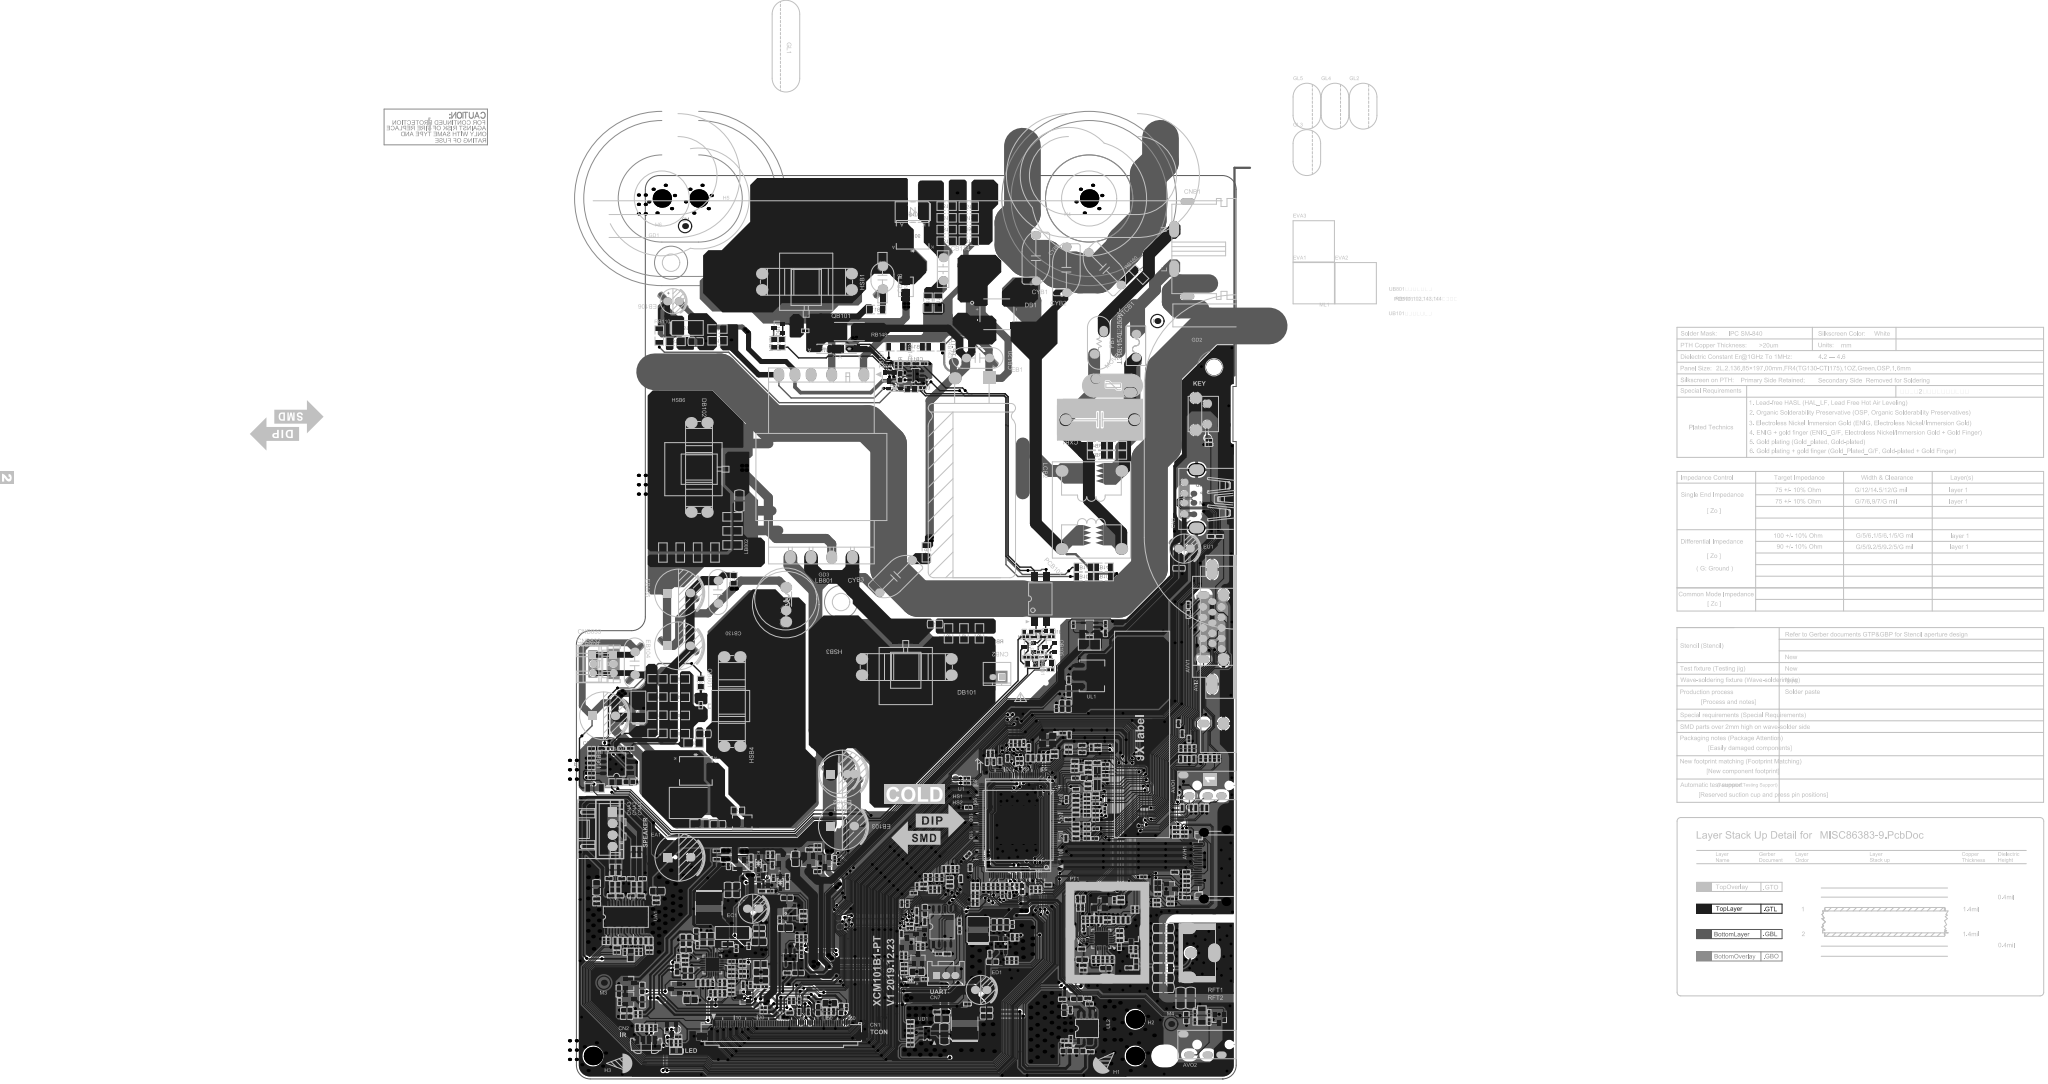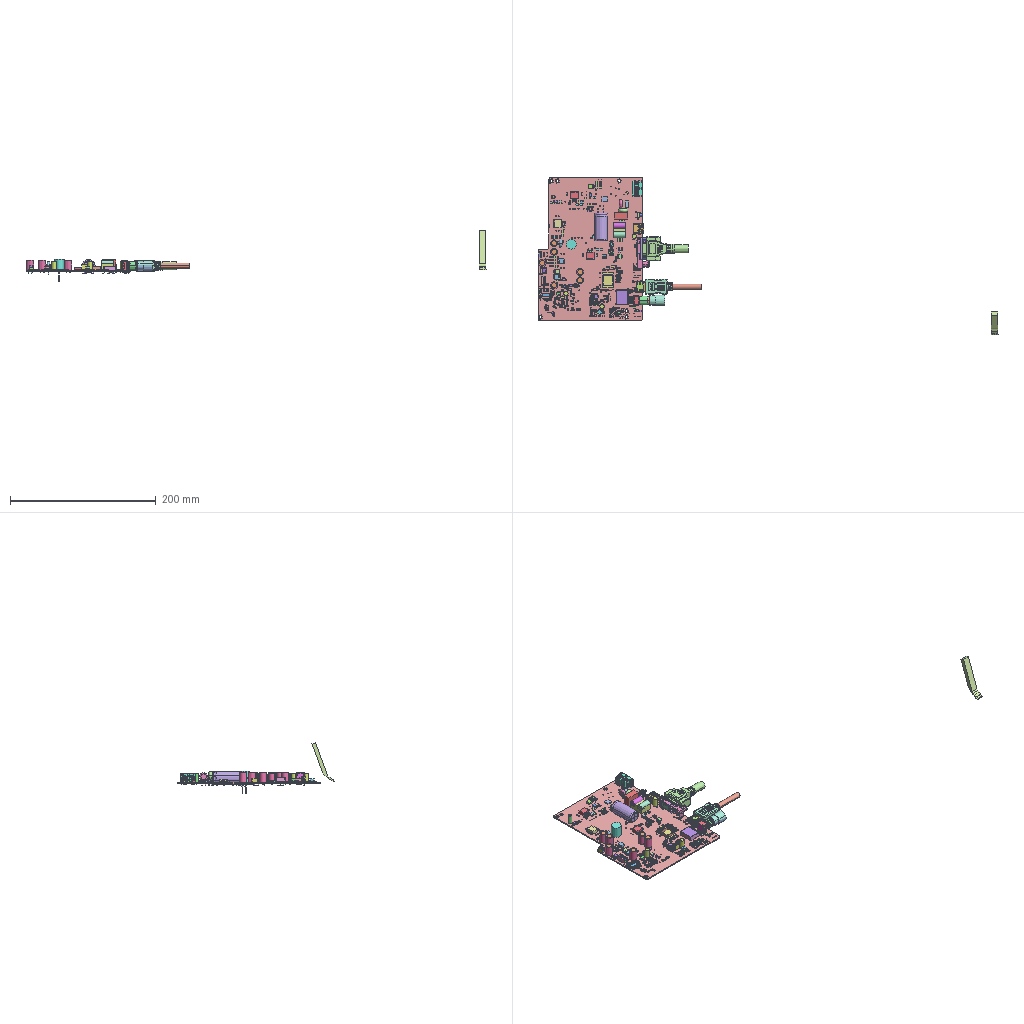Circuit board layout | Altium Designer | box 631.6 x 216.7 x 69.7 mm
Part placement, first 370 of 744 lines:
Designator,Comment,Layer,Footprint,Center-X(mm),Center-Y(mm),Rotation
ML1,NC/Mylar sheet,XXXXXXXXXXXXXXX,(85+6)×(123.5+6)×0.43mm,SE42B,black,TopLayer,Mylar,-883.787,-746.906,90
EVA6,NC/7×7×3mm-C-4305 fire-retardant foam-black,BottomLayer,EVA(7*7*3),-883.787,-746.906,180
EVA5,NC/7×7×3mm-C-4305 fire-retardant foam-black,BottomLayer,EVA(7*7*3),-883.787,-746.906,180
EVA4,NC/7×7×3mm-C-4305 fire-retardant foam-black,BottomLayer,EVA(7*7*3),-883.787,-746.906,180
RV23,NC/Thick film resistor,RES,1/16W,0ohm,±1%,0402,SMD,TopLayer,R0402,-3.759,69.901,90
RV22,NC/Thick film resistor,RES,1/16W,0ohm,±1%,0402,SMD,TopLayer,R0402,-5.69,69.901,90
DK2,NC/TVS diode,DIO ESD,3pF,58V,0402,SMD,SDV1005H260C030YPTF,Sunlord,TopLayer,DIODE-S0402,-14.275,38.151,180
CVBS_IN/OUT,TEST,BottomLayer,TP,-10.108,59.398,90
OE1,TEST,BottomLayer,TP,-86.335,33.172,180
RC36,Thick film resistor,RES,1/16W,10ohm,±1%,0402,SMD,TopLayer,R0402,-99.365,34.747,270
RG5,Thick film resistor,RES,1/16W,0ohm,±1%,0402,SMD,TopLayer,R0402,-129.692,14.097,270
H5,Location hole,TopLayer,ASSE4.0C-3,-117.05,191.85,0
CT5,NC/10uF-0603-X5R-±20%-6.3V,TopLayer,C0603,-33.517,26.012,360
H6,Location hole,TopLayer,ASSE4.0C-3,-125.05,191.85,0
UR1,NC/SGM810-SXN3L,TopLayer,SO-23-1,-68.801,31.533,90
RV21,Thick film resistor,RES,1/16W,0ohm,±1%,0402,SMD,TopLayer,R0402,-60.223,34.29,90
RV20,Thick film resistor,RES,1/16W,0ohm,±1%,0402,SMD,TopLayer,R0402,-60.198,32.41,90
RR6,NC/0ohm-0402-±5%-1/16W,TopLayer,R0402,-72.847,31.598,270
RR5,NC/0ohm-0402-±5%-1/16W,TopLayer,R0402,-69.207,28.84,270
RR2,NC/100Kohm-0402-±5%-1/16W,TopLayer,R0402,-71.044,33.757,360
RR1,NC/1Kohm-0402-±5%-1/16W,TopLayer,R0402,-71.044,32.842,180
RA38,NC/100Kohm-0402-±5%-1/16W,TopLayer,R0402,-72.83,26.909,90
RA31,NC/NC/470Kohm-0402-±5%-1/16W,TopLayer,R0402,-67.759,21.754,180
RA19,NC/33Kohm-0402-±5%-1/16W,TopLayer,R0402,-72.28,24.98,180
RA18,NC/33Kohm-0402-±5%-1/16W,TopLayer,R0402,-72.28,23.125,180
RA16,NC/2Kohm-0402-±1%-1/16W,TopLayer,R0402,-72.28,24.04,360
RA10,NC/2K2ohm-0402-±5%-1/16W,TopLayer,R0402,-71.89,26.897,90
QA3,NC/LMBT3904LT1G,TopLayer,SOT-23,-71.696,29.704,180
QA2,NC/LMBT3906LT1G,TopLayer,SOT-23,-69.258,26.148,180
HS2,NC/Heat sink,15.0×15.0×5.0mm,AL1060H-24,black,high-emissivity paint,stamped with bend,no press-fit legs,YT,TopLayer,HS(15X15X5)-S,-883.787,-746.906,0
H3,Location hole,TopLayer,ASSE4.0C-3,-139.831,4.85,0
DV8,NC/SFI0402-240E-2R5PP-LF,TopLayer,DIODE-S0402,-17.29,37.952,360
DV7,NC/SFI0402-240E-2R5PP-LF,TopLayer,DIODE-S0402,-17.306,38.969,360
DV6,NC/SFI0402-240E-2R5PP-LF,TopLayer,DIODE-S0402,-6.655,69.901,270
DV5,NC/SFI0402-240E-2R5PP-LF,TopLayer,DIODE-S0402,-4.724,69.901,270
DR1,NC/AVLC18S02003,TopLayer,DIODE-S0402,-59.957,43.612,90
CV23,NC/33pF-0402-NPO-±5%-50V,TopLayer,C0402,-11.748,75.285,270
CV22,NC/33pF-0402-NPO-±5%-50V,TopLayer,C0402,-12.56,77.47,270
CV21,NC/33pF-0402-NPO-±5%-50V,TopLayer,C0402,-10.44,101.289,270
CV20,NC/33pF-0402-NPO-±5%-50V,TopLayer,C0402,-9.195,69.781,90
CV19,NC/33pF-0402-NPO-±5%-50V,TopLayer,C0402,-9.155,72.056,90
CT2,10uF-0603-X5R-±20%-6.3V,TopLayer,C0603,-28.386,24.132,180
CR1,NC/1uF-0402-X5R-±20%-16V,TopLayer,C0402,-68.191,28.866,270
CO77,NC/10uF-0603-X5R-±20%-6.3V,TopLayer,C0603,-10.846,13.365,270
CA36,NC/10uF-0805-X5R-±20%-16V,TopLayer,C0805,-69.448,23.398,360
RT78,NC/,TopLayer,R0402SC,-33.419,37.384,90
RT77,NC/,TopLayer,R0402SC,-34.337,37.384,90
CT71,NC/30pF-0402-NPO-±5%-50V,TopLayer,C0402,-33.266,39.229,270
CT70,NC/30pF-0402-NPO-±5%-50V,TopLayer,C0402,-34.52,39.205,90
CF5,NC/0ohm-0402-PCB,TopLayer,R0402SC,-25.11,39.563,180
CF14,NC/4.7pF-0402-NPO-±5%-50V,TopLayer,C0402,-25.11,38.547,180
LF1,1000pF-0402-X7R-±10%-50V,TopLayer,L0402,-26.52,38.966,90
CT15,NC/8pF-0402-NPO-±5%-50V,TopLayer,C0402,-30.414,34.711,270
CT14,NC/8pF-0402-NPO-±5%-50V,TopLayer,C0402,-31.379,34.736,90
YT1,NC/Passive standard-package crystal oscillator,SPXO,24MHz,±20ppm,16pF,3.2×2.5,SMD,SMD3225 24.000MHZ,JWT,TopLayer,XTAL-S-10,-29.758,38.102,360
RT18,Thick film resistor,RES,1/16W,10Kohm,±1%,0402,SMD,TopLayer,R0402,-32.344,34.724,90
RT11,Thick film resistor,RES,1/16W,1.8Kohm,±1%,0402,SMD,TopLayer,R0402,-26.642,34.699,270
RT6,Thick film resistor,RES,1/16W,33ohm,±1%,0402,SMD,TopLayer,R0402,-21.581,36.946,90
RT5,Thick film resistor,RES,1/16W,33ohm,±1%,0402,SMD,TopLayer,R0402,-22.496,36.946,90
RT2,Thick film resistor,RES,1/16W,100ohm,±1%,0402,SMD,TopLayer,R0402,-33.258,34.736,90
LT12,Ferrite bead,BEAD,120ohm,0402,800mA,SMD,TP,CBM100505U121T,FH,TopLayer,L0402,-33.263,23.726,360
LT11,NC/SDCL1005CR27JTDF(Sunlord),TopLayer,L0402,-22.146,26.838,180
LT10,SDCL1005CR18JTDF(180nH-0402±5%-C),TopLayer,L0402,-25.346,31.282,360
LT9,NC/SDCL1608CR22JT(F),TopLayer,L0603,-21.75,25.04,270
LT8,GZ1005U102CTF(1000ohm-300mA),TopLayer,L0402,-25.346,30.177,360
LT6,GZ1005U102CTF(1000ohm-300mA),TopLayer,L0402,-25.435,28.818,270
LT3,Thick film resistor,RES,1/16W,0ohm,±1%,0402,SMD,TopLayer,L0402,-22.907,28.272,90
LT2,GZ1005U102CTF(1000ohm-300mA),TopLayer,L0402,-29.029,26.062,270
LT1,Multilayer inductor,HF Inductor,68nH,±5%,0402,SMD,SDCL1005C68NJTDF,Sunlord,TopLayer,L0402,-28.064,26.062,90
DT1,Switching diode,DIO SW D2,200mA,100V,SOT-23,SMD,BAV99,YJ,TopLayer,SO-23,-22.839,30.813,360
CT29,6800pF-0402-X7R-±10%-50V,TopLayer,C0402,-28.026,35.13,360
CT27,Ceramic capacitor,CAP MC,16V,0.1uF,±10%,X7R,0402,SMD,TP,TopLayer,C0402,-29.436,34.698,90
CT26,330pF-0402-NPO-±5%-50V,TopLayer,C0402,-28.026,34.203,360
CT25,Ceramic capacitor,CAP MC,16V,0.1uF,±10%,X7R,0402,SMD,TP,TopLayer,C0402,-25.677,34.648,90
CT21,0.047uF-0402-X7R-±10%-16V,TopLayer,C0402,-25.372,32.348,360
CT18,Ceramic capacitor,CAP MC,16V,0.1uF,±10%,X7R,0402,SMD,TP,TopLayer,C0402,-33.614,28.323,360
CT17,NC/180pF-0402-NPO-±5%-50V,TopLayer,C0402,-23.374,24.216,180
CT13,NC/1.2pF-0402-NPO-±0.25pf-50V,TopLayer,C0402,-21.831,28.24,90
CT12,0.022uF-0402-X7R-±10%-16V,TopLayer,C0402,-31.067,26.062,270
CT11,0.022uF-0402-X7R-±10%-16V,TopLayer,C0402,-29.987,26.063,90
CT9,Ceramic capacitor,CAP MC,16V,0.1uF,±10%,X7R,0402,SMD,TP,TopLayer,C0402,-26.997,26.062,270
CT8,Ceramic capacitor,CAP MC,50V,22pF,±5%,NPO,0402,SMD,TP,TopLayer,C0402,-23.53,34.648,270
CT7,Ceramic capacitor,CAP MC,50V,22pF,±5%,NPO,0402,SMD,TP,TopLayer,C0402,-24.597,34.648,270
CT6,Ceramic capacitor,CAP MC,16V,0.1uF,±10%,X7R,0402,SMD,TP,TopLayer,C0402,-33.289,24.767,180
CT1,Ceramic capacitor,CAP MC,16V,0.1uF,±10%,X7R,0402,SMD,TP,TopLayer,C0402,-33.225,32.933,90
UT1,Silicon tuner IC,IC Si Tuner,QFN24,SMD,R842,Rafael,TopLayer,QFN24/0.5-3,-29.36,30.57,180
RT9,NC/430ohm-0402-±5%-1/16W,TopLayer,R0402,-31.534,72.238,90
RT8,NC/,TopLayer,R0402SC,-30.163,72.721,180
RT7,NC/,TopLayer,R0402SC,-30.163,71.794,180
CT24,30pF-0402-NPO-±5%-50V,TopLayer,C0402,-33.521,72.721,180
CT23,Ceramic capacitor,CAP MC,16V,0.1uF,±10%,X7R,0402,SMD,TP,TopLayer,C0402,-36.487,72.371,180
CT20,Ceramic capacitor,CAP MC,16V,0.1uF,±10%,X7R,0402,SMD,TP,TopLayer,C0402,-36.487,71.26,180
CT10,30pF-0402-NPO-±5%-50V,TopLayer,C0402,-33.521,71.184,360
5V_STB,TEST,BottomLayer,TP,-74.651,18.466,90
RG62,Thick film resistor,RES,1/16W,0ohm,±1%,0402,SMD,TopLayer,R0402,-69.469,41.986,270
RG60,NC/33ohm-0402-±5%-1/16W,TopLayer,R0402,-58.611,64.529,180
RG59,Thick film resistor,RES,1/16W,0ohm,±1%,0402,SMD,TopLayer,R0402,-70.18,40.538,180
RG15,12Kohm-0402-±1%-1/16W,TopLayer,R0402,-121.405,26.307,270
RG14,Thick film resistor,RES,1/16W,3Kohm,±1%,0402,SMD,TopLayer,R0402,-113.925,20.955,90
RG13,Thick film resistor,RES,1/16W,39Kohm,±1%,0402,SMD,TopLayer,R0402,-109.839,25.618,180
RG12,NC/Thick film resistor,RES,1/16W,10Kohm,±1%,0402,SMD,TopLayer,R0402,-95.123,14.599,270
CG22,NC/1uF-0603-X5R-±10%-50V,TopLayer,C0603,-103.81,31.521,360
Y1,Passive crystal oscillator,SPXO,24MHz,±10ppm,12pF,SMD3225,SMD,SX32Y024000BC1T-Z,TKD,TopLayer,XTAL-S-3,-41.006,73.97,180
XCM101B1-PT,PCB_NAME,TopLayer,PCB_NAME,-76.708,16.002,180
VON,TEST,BottomLayer,TP,-124.904,17.221,180
VOFF,TEST,BottomLayer,TP,-104.623,16.205,180
VMID/SDA,TEST,BottomLayer,TP,-61.151,65.532,90
VMID/SCL,TEST,BottomLayer,TP,-58.814,64.529,180
USB_5V,TEST,BottomLayer,TP,-9.31,123.13,180
USB0_DP,TEST,BottomLayer,TP,-9.31,127.63,180
USB0_DM,TEST,BottomLayer,TP,-9.31,125.63,180
UL3,LDO IC,IC LDO,0.3A,3.3V,6V,SOT23-5,SMD,LC1463CB5ATR33,Leadchip,TopLayer,SOP23-5-1,-97.079,26.454,180
UC4,Operational amplifier,AMP,1,9MHz,SOT-23-5,SMD,SGM8425AYN5G/TR,SGMICRO,TopLayer,SOT-23-5,-97.079,36.411,360
UC2,Tcon driver IC,IC Tcon  Driver,VQFN-24L,SMD,ANX6732AAQX,ANAX,TopLayer,QFN24/0.5-5,-114.014,24.973,360
UC1,Regulator IC,IC Regulator,2.50V,0.4%,SOT-23,SMD,BR431M-A,Blue Rocket,TopLayer,SO-23-1,-107.112,17.843,90
TVCOM,TEST,BottomLayer,TP,-96.203,15.989,180
TP,TEST,BottomLayer,TP,-92.786,12.357,180
SK1,Tact switch,Tact Switch,160±50gf,7.0×10.3×7.0mm,DIP,106520070,VAST,TopLayer,KEY-HD-6,-7.6,145,90
RM12,Thick film resistor,RES,1/16W,100Kohm,±1%,0402,SMD,TopLayer,R0402,-102.565,45.999,90
RL51,Thick film resistor,RES,1/16W,10Kohm,±1%,0402,SMD,TopLayer,R0402,-94.64,30.632,270
RL50,NC/10Kohm-0402-±5%-1/16W,TopLayer,R0402,-94.628,28.892,90
RL7,Thick film resistor,RES,1/16W,4.7Kohm,±1%,0402,SMD,TopLayer,R0402,-93.726,30.632,270
RL3,NC/Thick film resistor,RES,1/16W,4.7Kohm,±5%,0402,SMD,TopLayer,R0402,-95.555,30.632,270
RGV1,NC/0ohm-0402-±5%-1/16W,TopLayer,R0402,-71.564,38.227,270
RG78,NC/0ohm-0402-PCB,TopLayer,R0402SC,-72.784,38.227,270
RG48,Thick film resistor,RES,1/16W,0ohm,±1%,0402,SMD,TopLayer,R0402,-102.616,20.117,360
RG46,NC/0ohm-0402-±5%-1/16W,TopLayer,R0402,-66.523,41.3,270
RG43,Thick film resistor,RES,1/16W,0ohm,±1%,0402,SMD,TopLayer,R0402,-97.257,17.031,270
RG41,NC/0ohm-0402-±5%-1/16W,TopLayer,R0402,-84.823,15.672,270
RG39,Thick film resistor,RES,1/16W,0ohm,±1%,0402,SMD,TopLayer,R0402,-89.56,14.707,90
RG26,NC/0ohm-0402-PCB,TopLayer,R0402SC,-64.694,41.3,270
RG25,NC/0ohm-0402-±5%-1/16W,TopLayer,R0402,-68.047,41.478,180
RC35,10Kohm-0402-±1%-1/16W,TopLayer,R0402,-94.209,34.493,360
RC33,NC/0ohm-0402-±5%-1/16W,TopLayer,R0402,-102.845,14.63,360
RC32,Thick film resistor,RES,1/16W,0ohm,±1%,0402,SMD,TopLayer,R0402,-102.845,15.545,180
RC31,10Kohm-0402-±1%-1/16W,TopLayer,R0402,-94.221,36.551,180
RC27,Thick film resistor,RES,1/16W,47Kohm,±1%,0402,SMD,TopLayer,R0402,-130.683,14.097,270
RC24,Thick film resistor,RES,1/16W,10Kohm,±1%,0402,SMD,TopLayer,R0402,-119.507,18.694,180
RC23,NC/0ohm-0402-±5%-1/16W,TopLayer,R0402,-134.212,16.803,270
RC20,Thick film resistor,RES,1/16W,0ohm,±1%,0402,SMD,TopLayer,R0402,-113.055,49.733,180
RC19,NC/0ohm-0402-±5%-1/16W,TopLayer,R0402,-113.055,47.904,360
RC18,Thick film resistor,RES,1/16W,47Kohm,±1%,0402,SMD,TopLayer,R0402,-106.096,29.02,90
RC15,Thick film resistor,RES,1/16W,47Kohm,±1%,0402,SMD,TopLayer,R0402,-109.884,23.385,360
RC14,Thick film resistor,RES,1/16W,4.7ohm,±1%,0402,SMD,TopLayer,R0402,-109.88,20.304,360
RC13,Thick film resistor,RES,1/16W,51Kohm,±1%,0402,SMD,TopLayer,R0402,-109.884,24.401,360
RC12,Thick film resistor,RES,1/16W,33Kohm,±1%,0402,SMD,TopLayer,R0402,-109.884,22.471,180
RC10,Thick film resistor,RES,1/16W,100Kohm,±1%,0402,SMD,TopLayer,R0402,-109.893,19.393,360
RC8,NC/0ohm-0402-PCB,TopLayer,R0402SC,-119.945,24.948,360
RC4,NC/0ohm-0402-PCB,TopLayer,R0402SC,-107.29,20.523,90
RC3,Thick film resistor,RES,1/16W,1.8Kohm,±1%,0402,SMD,TopLayer,R0402,-105.715,20.523,270
RC2,12Kohm-0402-±1%-1/16W,TopLayer,R0402,-104.343,20.117,360
RC1,33ohm-0805-±5%-1/8W,TopLayer,R0805,-103.53,25.044,180
QM7,MOSFET,PMOS,-4.3A,-30V,0.048ohm@ID=-3A@VGS=-4.5V,SOT-23-3L,NCE3407AY,NCEPOWER,TopLayer,SOT-23-1,-108.013,46.532,360
POL,TEST,BottomLayer,TP,-94.767,12.383,180
NO DOLBY,NO DOLBY,BottomLayer,NO_DOLBY-SILK,-883.787,-746.906,180
LC1,Power inductor,Power Inductor,10uH,±10%,2A,0.3×1P,DR5.8×4.5,SMD,CKO54-10uH/K,CK,TopLayer,L(5.8*4.5)-S,-114.795,37.224,90
GREF,TEST,BottomLayer,TP,-92.024,15.926,180
EC1,Aluminium electrolytic capacitor,CAP AL,35V,100uF,±20%,LD,KF,P,2.5mm,6.3×11,DIP,TP,CapXon,TopLayer,EC(6.3*11)-V-2.5,-105.219,36.678,360
DM3,NC/Switching diode,DIO SW S,150mA,75V,SOD-323,SMD,1N4148WS,YJ,TopLayer,DIODE-S-12,-103.988,46.977,270
DK20,WEJT61RC-871-red,TopLayer,DIODE-S0603,-121.906,6.094,360
DC4,Switching diode,DIO SW D2,200mA,100V,SOT-23,SMD,BAV99,YJ,TopLayer,SO-23,-132.014,17.368,90
DC3,Switching diode,DIO SW D2,200mA,100V,SOT-23,SMD,BAV99,YJ,TopLayer,SO-23,-132.002,20.816,90
DC2,Switching diode,DIO SW D2,200mA,100V,SOT-23,SMD,BAV99,YJ,TopLayer,SO-23,-122.092,19.704,270
DC1,Schottky diode,DIO SBD S,1A,40V,DO-214AC,SMD,SS14W,WILLAS,TopLayer,DIODE-S-1,-109.576,31.826,360
CU6,NC/0ohm-0402-PCB,TopLayer,R0402SC,-53.95,70.907,270
CU5,NC/0ohm-0402-PCB,TopLayer,R0402SC,-53.035,70.907,270
CPV,TEST,BottomLayer,TP,-71.044,33.236,180
CPV2,TEST,BottomLayer,TP,-85.001,12.383,180
CN2,IR receiver transistor,IR Receriver,2.7-5.5V,37.9KHz,SMD,SIRAB39R1,SL,TopLayer,REMOTE-HS-1,-128.4,8.505,0
CN1,FFC connector,FFC connector,60Pin,D0.5,Bottom,lock,SMD,0.5-22-60PBX-P,XFE,TopLayer,FFC60H/0.5S-11,-99,10.727,360
CM11,Ceramic capacitor,CAP MC,16V,0.22uF,±20%,X5R,0402,SMD,TP,TopLayer,C0402,-105.588,48.197,90
CM10,NC/0.022uF-0402-X7R-±10%-50V,TopLayer,C0402,-105.55,46.304,90
CL16,Ceramic capacitor,CAP MC,16V,0.1uF,±10%,X7R,0402,SMD,TP,TopLayer,C0402,-94.615,27.114,270
CG16,Ceramic capacitor,CAP MC,50V,33pF,±5%,NPO,0402,SMD,TP,TopLayer,C0402,-108.814,28.435,90
CC51,1uF-0402-X5R-±20%-6.3V,TopLayer,C0402,-97.739,23.114,360
CC50,NC/10uF-0603-X5R-±20%-6.3V,TopLayer,C0603,-95.352,23.114,360
CC43,10uF-0805-X5R-±20%-16V,TopLayer,C0805,-98.12,32.982,180
CC42,Ceramic capacitor,CAP MC,16V,0.1uF,±10%,X7R,0402,SMD,TP,TopLayer,C0402,-94.208,35.496,360
CC38,Ceramic capacitor,CAP MC,50V,0.1uF,±10%,X7R,0603,SMD,TP,TopLayer,C0603,-97.777,39.484,180
CC34,Ceramic capacitor,CAP MC,50V,0.1uF,±10%,X7R,0603,SMD,TP,TopLayer,C0603,-132.651,13.614,360
CC33,1uF-0603-X5R-±10%-50V,TopLayer,C0603,-132.639,15.011,360
CC32,NC/33pF-0402-NPO-±5%-50V,TopLayer,C0402,-113.392,18.669,270
CC31,Ceramic capacitor,CAP MC,50V,0.1uF,±10%,X7R,0603,SMD,TP,TopLayer,C0603,-129.235,16.815,90
CC30,NC/10uF-0805-X5R-±20%-16V,TopLayer,C0805,-118.77,17.259,360
CC29,10uF-0805-X5R-±20%-16V,TopLayer,C0805,-88.468,16.485,360
CC27,Ceramic capacitor,CAP MC,50V,0.1uF,±10%,X7R,0603,SMD,TP,TopLayer,C0603,-129.235,19.761,270
CC26,NC/33pF-0402-NPO-±5%-50V,TopLayer,C0402,-111.36,18.669,270
CC25,NC/33pF-0402-NPO-±5%-50V,TopLayer,C0402,-107.449,25.645,360
CC24,Ceramic capacitor,CAP MC,16V,0.1uF,±10%,X7R,0402,SMD,TP,TopLayer,C0402,-117.129,20.937,270
CC23,NC/0.1uF-0402-X5R-±20%-16V,TopLayer,C0402,-107.444,22.396,180
CC21,Ceramic capacitor,CAP MC,50V,1000pF,±10%,X7R,0402,SMD,TP,TopLayer,C0402,-107.444,23.463,360
CC20,Ceramic capacitor,CAP MC,25V,1uF,±10%,X7R,0603,SMD,TP,TopLayer,C0603,-103.81,32.944,360
CC19,Ceramic capacitor,CAP MC,25V,10uF,±10%,X5R,0805,SMD,TP,TopLayer,C0805,-103.835,29.909,360
CC18,1uF-0402-X5R-±20%-6.3V,TopLayer,C0402,-109.884,21.302,180
CC17,1uF-0402-X5R-±20%-6.3V,TopLayer,C0402,-111.36,20.955,90
CC15,1uF-0402-X5R-±20%-6.3V,TopLayer,C0402,-114.98,20.955,270
CC13,NC/0.1uF-0402-X5R-±20%-16V,TopLayer,C0402,-110.503,46.495,270
CC12,NC/Ceramic capacitor,CAP MC,16V,10uF,±20%,X5R,0805,SMD,TP,TopLayer,C0805,-110.582,41.219,90
CC11,Ceramic capacitor,CAP MC,50V,0.1uF,±10%,X7R,0603,SMD,TP,TopLayer,C0603,-119.698,28.092,180
CC10,Ceramic capacitor,CAP MC,50V,0.1uF,±10%,X7R,0603,SMD,TP,TopLayer,C0603,-120.421,30.226,90
CC9,NC/0.1uF-0603-X7R-±10%-50V,TopLayer,C0603,-118.999,30.226,90
CC8,Ceramic capacitor,CAP MC,16V,10uF,±20%,X5R,0805,SMD,TP,TopLayer,C0805,-108.753,41.219,90
CC7,Ceramic capacitor,CAP MC,50V,0.1uF,±10%,X7R,0603,SMD,TP,TopLayer,C0603,-120.053,23.05,270
CC5,Ceramic capacitor,CAP MC,16V,2.2uF,±10%,X5R,0603,SMD,TP,TopLayer,C0603,-121.672,23.919,270
CC4,Ceramic capacitor,CAP MC,25V,1uF,±10%,X7R,0603,SMD,TP,TopLayer,C0603,-118.681,23.05,90
CC2,Ceramic capacitor,CAP MC,25V,10uF,±10%,X5R,0805,SMD,TP,TopLayer,C0805,-103.454,23.312,180
CC1,NC/Ceramic capacitor,CAP MC,25V,10uF,±10%,X5R,0805,SMD,TP,TopLayer,C0805,-103.454,21.483,180
3V3_TUNER,TEST,BottomLayer,TP,-35.821,19.686,90
COLD,COLD,TopLayer,COLD,-883.787,-746.906,360
AI_V,AI_GRIPPER_V,TopLayer,AI_GRIPPER_V,483.311,-17.234,270
UART_RX,TEST,BottomLayer,TP,-12.135,56.667,90
CN7,Connector socket,connect jack,3Pin,D2.0,D,SNAP,L=2.8mm,DIP,CNJST,TopLayer,SIP3/2.0D-3,-63.195,22.555,360
UU1,NC/Current limit switch,IC OCP,0.4-2A adj,5.5V,H,SOT23-5,SMD,SY6280AAAC,SILERGY,TopLayer,SOP23-5-1,-31.902,98.527,90
RU45,NC/Thick film resistor,RES,1/16W,5.6Kohm,±1%,0402,SMD,TopLayer,R0402,-28.448,99.187,90
RU4,NC/Thick film resistor,RES,1/16W,4.7Kohm,±1%,0402,SMD,TopLayer,R0402,-35.433,99.06,270
LBA8,NC/0ohm-0603-PCB,TopLayer,R0603SC,-129.899,49.489,90
LBA7,NC/0ohm-0603-PCB,TopLayer,R0603SC,-131.118,49.489,90
LBA6,NC/0ohm-0603-PCB,TopLayer,R0603SC,-134.42,45.578,90
LBA5,NC/0ohm-0603-PCB,TopLayer,R0603SC,-135.791,45.578,90
FU1,NC/NSMD110(1206-1.1A),TopLayer,FUSE1.1A-S,-31.953,94.717,180
DV3,NC/NC/AVLC18S02003,TopLayer,DIODE-S0402,-11.26,53.861,180
CH15,NC/1uF-0402-X5R-±20%-16V,TopLayer,C0402,-13.373,45.072,180
CT40,Ceramic capacitor,CAP MC,1KV,470pF,±5%,NPO,1206,SMD,TP,TopLayer,C1206,-15.849,24.193,180
CT41,Ceramic capacitor,CAP MC,1KV,4700pF,±10%,X7R,1206,SMD,TP,TopLayer,C1206,-15.85,26.378,360
CT42,Ceramic capacitor,CAP MC,1KV,4700pF,±10%,X7R,1206,SMD,TP,TopLayer,C1206,-15.863,22.022,360
CT43,Ceramic capacitor,CAP MC,1KV,4700pF,±10%,X7R,1206,SMD,TP,TopLayer,C1206,-15.85,19.875,360
CT44,Ceramic capacitor,CAP MC,1KV,4700pF,±10%,X7R,1206,SMD,TP,TopLayer,C1206,-15.85,28.511,360
CT45,Ceramic capacitor,CAP MC,1KV,4700pF,±10%,X7R,1206,SMD,TP,TopLayer,C1206,-12.09,17.628,90
CT46,Ceramic capacitor,CAP MC,1KV,4700pF,±10%,X7R,1206,SMD,TP,TopLayer,C1206,-15.85,30.709,360
CT47,NC/Ceramic capacitor,CAP MC,1KV,4700pF,±10%,X7R,1206,SMD,TP,TopLayer,C1206,-9.906,17.628,90
CT48,NC/Ceramic capacitor,CAP MC,1KV,4700pF,±10%,X7R,1206,SMD,TP,TopLayer,C1206,-15.85,32.893,360
PT1,20.3×16.3×6-LHD (with seal),TopLayer,SHIELD(16*20*6),-28.026,31.897,360
DT2,NC/AVLC18S02003,TopLayer,DIODE-S0402,-45.148,72.288,90
DT3,NC/AVLC18S02003,TopLayer,DIODE-S0402,-46.215,73.19,90
??U1?,Glue,0.1g,silicone,ZJ,TopLayer,Heat-Shrinkable_Tube,1.429,25.711,90
VCC_PANEL,TEST,BottomLayer,TP,-108.788,50.102,0
UL2,LDO IC,IC LDO,1A,3.3V+ADJ,12V,ESOP-8,SMD,LC1118CS8TRAD33,Leadchip,TopLayer,SOP8/1.27-3,-32.461,11.024,90
UL1,LDO IC,IC LDO,1A,1.8V,15V,SOT-223,SMD,SCJT1117B-1.8V,CJKJ,TopLayer,SOT-223,-31.413,87.898,270
UD2,DC-DC IC,IC DCDC,Syn,1.2A,6.0V,1.5MHz,SOT23-5,SMD,TMI3408,TOLL,TopLayer,SOT-23-5,-51.199,29.132,180
UD1,DC-DC IC,IC DC-DC,Syn,2A,18V,600KHz,SOT23-6,SMD,TMI3252T,TOLL,TopLayer,TSOT23-6,-67.259,9.957,180
UART_TX,TEST,BottomLayer,TP,-12.954,54.419,90
UA1,Audio amplifier IC,Class D,2×10W@13V@8ohm,HTSSOP-28,SMD,CS3817BEO,HRXK,TopLayer,SSOP28/0.65-5,-132.845,35.316,90
STV,TEST,BottomLayer,TP,-86.677,35.128,180
RV19,Thick film resistor,RES,1/16W,100ohm,±1%,0402,SMD,TopLayer,R0402,-56.348,40.162,270
RV18,Thick film resistor,RES,1/16W,100ohm,±1%,0402,SMD,TopLayer,R0402,-57.262,40.162,270
RV14,NC/10Kohm-0402-±5%-1/16W,TopLayer,R0402,-10.205,69.775,270
RV13,Thick film resistor,RES,1/16W,4.7Kohm,±1%,0402,SMD,TopLayer,R0402,-57.277,38.456,270
RV12,Thick film resistor,RES,1/16W,4.7Kohm,±1%,0402,SMD,TopLayer,R0402,-56.35,38.456,270
RV10,NC/100ohm-0402-±5%-1/16W,TopLayer,R0402,-11.119,69.775,270
RV6,NC/100ohm-0402-±5%-1/16W,TopLayer,R0402,-11.067,72.056,270
RV4,NC/10Kohm-0402-±5%-1/16W,TopLayer,R0402,-10.153,72.056,270
RPH2,Resistor array,RES ARRAY,1/16W,4×10Kohm,±5%,0402,SMD,TopLayer,RA0402,-17.056,42.164,180
RO10,NC/1Kohm-0402-±5%-1/16W,TopLayer,R0402,-5.893,14.321,270
RO9,NC/100ohm-0402-±5%-1/16W,TopLayer,R0402,-8.992,12.543,90
RO6,NC/10Kohm-0402-±5%-1/16W,TopLayer,R0402,-8.992,14.321,270
RO2,NC/100ohm-1206-±5%-1/4W,TopLayer,R1206,-7.468,13.813,90
RM10,Thick film resistor,RES,1/16W,4.7Kohm,±1%,0402,SMD,TopLayer,R0402,-101.422,40.958,360
RM8,Thick film resistor,RES,1/16W,4.7Kohm,±1%,0402,SMD,TopLayer,R0402,-103.2,40.958,180
RM7,Thick film resistor,RES,1/16W,47Kohm,±1%,0402,SMD,TopLayer,R0402,-100.711,43.853,90
RM6,NC/4K7ohm-0402-±5%-1/16W,TopLayer,R0402,-101.918,48.895,270
RM5,Thick film resistor,RES,1/16W,4.7Kohm,±1%,0402,SMD,TopLayer,R0402,-97.665,42.083,90
RM4,Thick film resistor,RES,1/16W,4.7Kohm,±1%,0402,SMD,TopLayer,R0402,-87.376,47.917,90
RM2,200Kohm-0402-±1%-1/16W,TopLayer,R0402,-91.059,49.962,180
RM1,Thick film resistor,RES,1/16W,4.7Kohm,±1%,0402,SMD,TopLayer,R0402,-91.072,50.902,180
RL5,91ohm-0402-±1%-1/16W,TopLayer,R0402,-37.37,8.306,180
RL4,150ohm-0402-±1%-1/16W,TopLayer,R0402,-35.992,8.687,270
RK21,Thick film resistor,RES,1/16W,510ohm,±1%,0402,SMD,TopLayer,R0402,-121.92,7.823,270
RK20,NC/10Kohm-0402-±5%-1/16W,TopLayer,R0402,-121.463,9.195,360
RK16,Thick film resistor,RES,1/16W,1Kohm,±1%,0402,SMD,TopLayer,R0402,-127.305,11.125,270
RK15,Thick film resistor,RES,1/16W,4.7Kohm,±1%,0402,SMD,TopLayer,R0402,-126.39,11.125,270
RK13,Thick film resistor,RES,1/16W,22ohm,±1%,0402,SMD,TopLayer,R0402,-129.316,11.166,270
RK6,1K2ohm-0402-±1%-1/16W,TopLayer,R0402,-5.944,139.294,180
RK1,NC/1K5ohm-0402-±5%-1/16W,TopLayer,R0402,-121.006,7.823,90
RI10,NC/SHORT,TopLayer,GND,-11.113,64.16,360
RH14,Thick film resistor,RES,1/16W,1Kohm,±1%,0402,SMD,TopLayer,R0402,-12.142,39.947,270
RH2,Thick film resistor,RES,1/16W,0ohm,±1%,0402,SMD,TopLayer,R0402,-11.277,52.901,360
RH1,Thick film resistor,RES,1/16W,0ohm,±1%,0402,SMD,TopLayer,R0402,-13.074,53.882,360
RG82,Thick film resistor,RES,1/10W,22ohm,±1%,0603,SMD,TopLayer,R0603,-110.655,29.401,180
RFT2,RF connector,RF JACK,H,IEC,T14.5,CH6.3,12.4×13.2×7.7mm,DIP,LHD-020 assembly,LHD,TopLayer,ANT-IEC14.5-H-4,-7.675,27.5,90
RFT1,NC/RF connector,RF JACK,H,F,T14.5,CH6.3,without pipe,12.4×13.2×7.7mm,DIP,LHD,TopLayer,T-13.2¡Á12.4¡Á7.7-F14.5,-7.675,27.5,90
RF14,NC/4K7ohm-0402-±5%-1/16W,TopLayer,R0402,-62.332,43.901,180
RF13,Thick film resistor,RES,1/16W,4.7Kohm,±1%,0402,SMD,TopLayer,R0402,-61.665,45.736,270
RD9,Thick film resistor,RES,1/16W,12Kohm,±1%,0402,SMD,TopLayer,R0402,-47.865,25.82,90
RD8,Thick film resistor,RES,1/16W,13Kohm,±1%,0402,SMD,TopLayer,R0402,-49.85,25.82,270
RD7,Thick film resistor,RES,1/16W,100Kohm,±1%,0402,SMD,TopLayer,R0402,-47.689,30.897,90
RD5,Thick film resistor,RES,1/16W,10.5Kohm,±1%,0402,SMD,TopLayer,R0402,-70.918,10.56,360
RD3,Thick film resistor,RES,1/16W,60.4Kohm,±1%,0402,SMD,TopLayer,R0402,-70.918,11.474,180
RD1,Thick film resistor,RES,1/16W,100Kohm,±1%,0402,SMD,TopLayer,R0402,-70.92,8.435,360
RA21,Thick film resistor,RES,1/16W,1Kohm,±1%,0402,SMD,TopLayer,R0402,-134.798,27.584,360
RA14,NC/0ohm-0402-±5%-1/16W,TopLayer,R0402,-132.946,30.084,90
RA12,NC/15Kohm-0402-±1%-1/16W,TopLayer,R0402,-129.598,27.696,90
RA11,NC/10Kohm-0402-±1%-1/16W,TopLayer,R0402,-130.512,27.696,90
RA8,Thick film resistor,RES,1/16W,4.7Kohm,±1%,0402,SMD,TopLayer,R0402,-136.657,30.103,90
RA5,Thick film resistor,RES,1/16W,1Kohm,±1%,0402,SMD,TopLayer,R0402,-127.728,27.602,360
RA4,NC/100Kohm-0402-±5%-1/16W,TopLayer,R0402,-133.048,27.696,270
RA3,Thick film resistor,RES,1/8W,10ohm,±1%,0805,SMD,TopLayer,R0805,-131.783,27.036,90
RA1,Thick film resistor,RES,1/16W,4.7Kohm,±1%,0402,SMD,TopLayer,R0402,-137.578,30.11,270
QO1,NC/General transistor,Dynatron,NPN,0.2A,40V,60-300,SOT-23,KMBT3904,KEXIN,TopLayer,SOT-23,-3.658,13.127,0
QM6,General transistor,Dynatron,NPN,0.2A,40V,30-300,SOT-23,LMBT3904LT1G,LRC,TopLayer,SOT-23,-102.895,43.218,180
QM5,MOSFET,PMOS,-4.4A,-30V,0.046ohm@ID=-4A@VGS=-4.5V,SOT-23,NCE3401AY,NCEPOWER,TopLayer,SOT-23-1,-98.54,47.956,180
QM2,General transistor,Dynatron,NPN,0.2A,40V,30-300,SOT-23,LMBT3904LT1G,LRC,TopLayer,SOT-23,-89.522,47.206,360
QM1,MOSFET,PMOS,-4.4A,-30V,0.046ohm@ID=-4A@VGS=-4.5V,SOT-23,NCE3401AY,NCEPOWER,TopLayer,SOT-23-1,-93.003,47.396,360
QK2,NC/MMBT3904(f=350MHz),TopLayer,SOT-23,-122.885,10.795,360
QH2,General transistor,Dynatron,NPN,0.2A,40V,30-300,SOT-23,LMBT3904LT1G,LRC,TopLayer,SOT-23,-14.25,41.471,90
LED,TEST,BottomLayer,TP,-121.73,10.808,270
LD2,Power inductor,Power Inductor,2.2uH,±20%,2A,0.28×1P,DR4.5×3.2,SMD,PIO43-2R2MTP02,FH,TopLayer,L(4.5*3.5)-S,-56.134,32.587,270
LD1,Power inductor,Power Inductor,4.7uH,±20%,2.8A,0.32×1P,DR5.8×4.5,SMD,PIO54-4R7MTP02,FH,TopLayer,L(5.8*4.5)-S,-59.106,12.04,270
LBA4,Ferrite bead,BEAD,600ohm,0603,2A,SMD,TP,EPZ1608E601-2R0TF,Sunlord,TopLayer,L0603,-129.848,41.818,90
LBA3,Ferrite bead,BEAD,600ohm,0603,2A,SMD,TP,EPZ1608E601-2R0TF,Sunlord,TopLayer,L0603,-131.123,41.818,90
LBA2,Ferrite bead,BEAD,600ohm,0603,2A,SMD,TP,EPZ1608E601-2R0TF,Sunlord,TopLayer,L0603,-134.47,41.818,90
LBA1,Ferrite bead,BEAD,600ohm,0603,2A,SMD,TP,EPZ1608E601-2R0TF,Sunlord,TopLayer,L0603,-135.791,41.818,90
KEY,TEST,BottomLayer,TP,-6.236,139.802,270
IR,TEST,BottomLayer,TP,-126.905,11.025,270
H2,Location hole,TopLayer,ASSE4.0C-3,-22.05,12.85,0
H1,Location hole,TopLayer,ASSE4.0C-3,-22.05,4.85,0
F2,Thick film resistor,RES,1/16W,0ohm,±1%,0402,SMD,TopLayer,R0402,-31.902,96.291,360
ED1,Aluminium electrolytic capacitor,CAP AL,10V,470uF,±20%,PKZH,P,2.5mm,6.3×11,DIP,TP,Koshin,TopLayer,EC(6.3*11)-V-2.5,-55.601,18.961,360
DV4,NC/NC/AVLC18S02003,TopLayer,DIODE-S0402,-13.074,54.847,360
DU4,NC/,TopLayer,DIODE-S0402,-3.624,118.307,180
DU3,NC/,TopLayer,DIODE-S0402,-5.504,118.305,360
DO3,NC/AVLC18S02003,TopLayer,DIODE-S0402,-6.401,59.08,90
DO2,NC/AVLC18S02003,TopLayer,DIODE-S0402,-11.786,59.08,90
DO1,NC/AVLC18S02003,TopLayer,DIODE-S0402,-8.788,59.08,90
DM1,NC/Switching diode,DIO SW S,150mA,75V,SOD-323,SMD,1N4148WS,BLUE ROCKET,TopLayer,DIODE-S-12,-99.225,42.799,270
DK6,NC/TVS diode,DIO ESD,0.5pF,25V,0402 DFN,SMD,AZ5325-01F.R7G,Amazing,TopLayer,DIODE-S0402,-58.522,16.332,360
DI5,NC/NC/AVLC18S02003,TopLayer,DIODE-S0402,-5.893,12.543,270
DI3,NC/AVLC18S02003,TopLayer,DIODE-S0402,-10.439,103.365,270
DI2,NC/AVLC18S02003,TopLayer,DIODE-S0402,-10.274,74.08,90
DI1,NC/AVLC18S02003,TopLayer,DIODE-S0402,-7.717,69.882,90
DH7,NC/NC/AVLC18S02003,TopLayer,DIODE-S0402,-10.821,42.182,360
DH6,NC/NC/AVLC18S02003,TopLayer,DIODE-S0402,-10.821,43.147,360
DH3,NC/NC/AVLC18S02003,TopLayer,DIODE-S0402,-10.821,44.112,360
DH2,NC/0ohm-0402-±5%-1/16W,TopLayer,DIODE-S0402,-13.074,52.916,360
CV10,NC/33pF-0402-NPO-±5%-50V,TopLayer,C0402,-12.084,69.775,270
CV9,NC/33pF-0402-NPO-±5%-50V,TopLayer,C0402,-12.032,72.056,270
CU2,Ceramic capacitor,CAP MC,6.3V,0.47uF,±10%,X5R,0402,SMD,TP,TopLayer,C0402,-28.448,97.286,90
CU1,NC/10uF-0603-X5R-±20%-6.3V,TopLayer,C0603,-12.446,111.379,180
CNA3,NC/Connector socket,connect jack,4Pin,D2.5,D,SNAP,Nature,L=2.8mm,DIP,W2411-04SVA-S03-E,XYDT,TopLayer,SIP4/2.5D-2,-135.814,54.415,270
CNA2,Connector socket,connect jack,4PIN,D2.50,L,SNAP,STEP,Fool-proofing,Nature,L=3.0mm,DIP,AMA,TopLayer,SIP4H/2.5D-7,-135.814,54.445,270
CNA1,NC/4PIN-2.54-D-H-G,TopLayer,SIP4/2.54D-1,-135.814,54.475,270
CN5,USB jack,USB Jack,USB2.0,H,Single,Black,flange,Block up,DIP,103411481,VAST,TopLayer,USB-HD-30,-9.96,126.5,90
CM7,0.022uF-0402-X7R-±10%-16V,TopLayer,C0402,-100.94,46.622,90
CM5,NC/10uF-0805-X5R-±20%-16V,TopLayer,C0805,-95.936,48.019,270
CM4,Ceramic capacitor,CAP MC,16V,0.1uF,±10%,X7R,0402,SMD,TP,TopLayer,C0402,-100.901,48.87,270
CM3,NC/Ceramic capacitor,CAP MC,16V,0.1uF,±10%,X7R,0402,SMD,TP,TopLayer,C0402,-97.665,43.963,270
CM2,Ceramic capacitor,CAP MC,16V,0.1uF,±10%,X7R,0402,SMD,TP,TopLayer,C0402,-91.122,45.212,360
CM1,0.22uF-0402-X5R-±10%-16V,TopLayer,C0402,-92.9,49.974,360
CL15,Ceramic capacitor,CAP MC,6.3V,1uF,±20%,X5R,0402,SMD,TP,TopLayer,C0402,-31.953,16.358,360
CL14,NC/10uF-0603-X5R-±20%-6.3V,TopLayer,C0603,-34.696,17.475,180
CL13,NC/Ceramic capacitor,CAP MC,16V,0.1uF,±10%,X7R,0402,SMD,TP,TopLayer,C0402,-32.309,17.577,360
CL12,Ceramic capacitor,CAP MC,6.3V,1uF,±20%,X5R,0402,SMD,TP,TopLayer,C0402,-36.068,15.011,90
CL11,NC/10uF-0603-X5R-±20%-6.3V,TopLayer,C0603,-37.389,14.986,270
CL10,NC/Ceramic capacitor,CAP MC,16V,0.1uF,±10%,X7R,0402,SMD,TP,TopLayer,C0402,-37.846,17.374,360
CL9,Ceramic capacitor,CAP MC,16V,0.1uF,±10%,X7R,0402,SMD,TP,TopLayer,C0402,-31.75,5.944,180
CL8,NC/10uF-0603-X5R-±20%-6.3V,TopLayer,C0603,-34.087,6.096,360
CL7,NC/10uF-0603-X5R-±20%-6.3V,TopLayer,C0603,-36.982,6.096,360
CL6,Ceramic capacitor,CAP MC,16V,0.1uF,±10%,X7R,0402,SMD,TP,TopLayer,C0402,-36.55,7.315,360
CL5,NC/10uF-0603-X5R-±20%-6.3V,TopLayer,C0603,-37.871,81.297,270
CL4,NC/10uF-0603-X5R-±20%-6.3V,TopLayer,C0603,-36.5,81.297,270
CL3,Ceramic capacitor,CAP MC,6.3V,1uF,±20%,X5R,0402,SMD,TP,TopLayer,C0402,-39.116,80.772,270
CL2,Ceramic capacitor,CAP MC,16V,0.1uF,±10%,X7R,0402,SMD,TP,TopLayer,C0402,-36.449,86.991,270
CL1,NC/10uF-0603-X5R-±20%-6.3V,TopLayer,C0603,-36.449,84.582,90
CK10,NC/0.1uF-0402-X5R-±20%-16V,TopLayer,C0402,-122.936,7.823,270
CK6,NC/10pF-0402-NPO-±5%-50V,TopLayer,C0402,-128.321,11.125,90
CK4,Ceramic capacitor,CAP MC,16V,0.1uF,±10%,X7R,0402,SMD,TP,TopLayer,C0402,-130.333,11.174,90
CI12,NC/4700pF-0402-X7R-±10%-50V,TopLayer,C0402,-9.804,59.08,270
CI11,NC/1000pF-0402-X7R-±10%-50V,TopLayer,C0402,-7.417,59.131,270
CH18,NC/0.1uF-0402-X7R-±10%-16V,TopLayer,C0402,-10.796,39.54,180
CH10,NC/30pF-0402-NPO-±5%-50V,TopLayer,C0402,-10.82,45.148,360